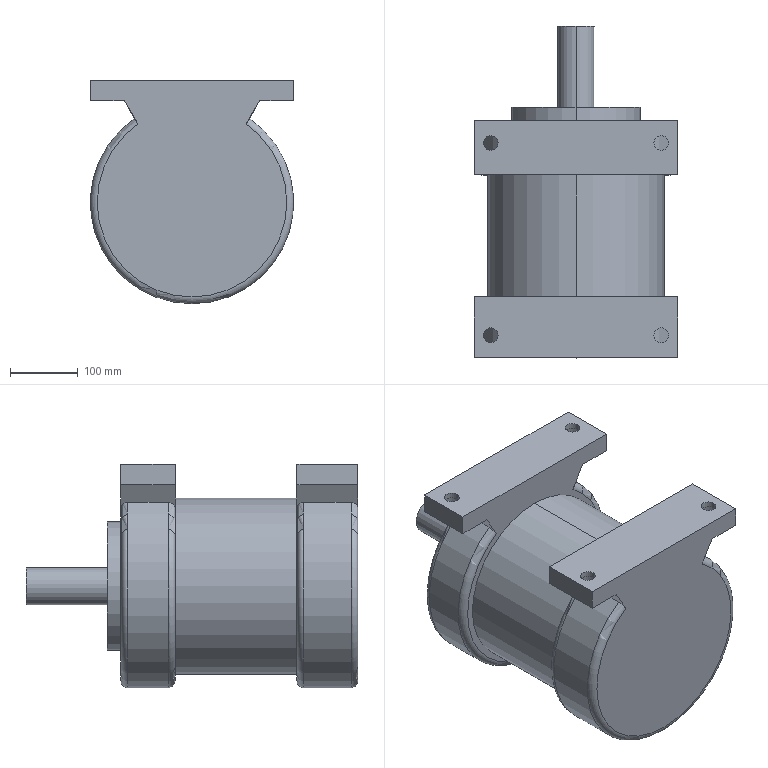Part | SolidWorks | features ICE 4, Extrusion 1, Fillet 1, HoleWzd 1 | 2 solids | 55 faces | box 300 x 490 x 330 mm | volume 24115520 mm3 | cylinder 26 | plane 25 | torus 4 | commonest cylinder face diameters 22 x8 33 x8 300 x4 55 x2 190 x2 260 x2